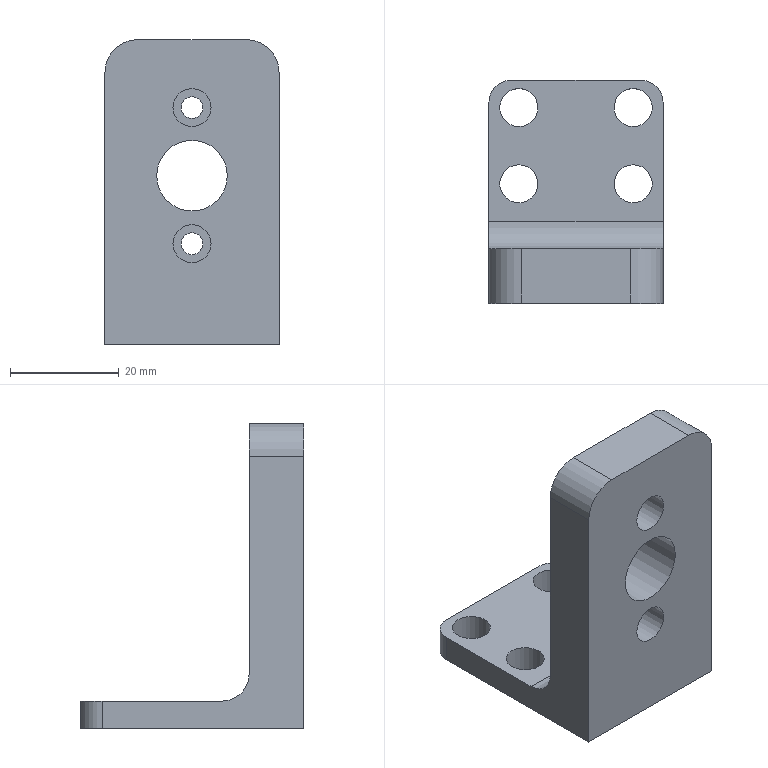Part | NX | features BREP 1, DATUM_CSYS 1 | 1 solid | 30 faces | box 32 x 41 x 56 mm | volume 19804 mm3 | cylinder 18 | plane 10 | cone 2 | commonest cylinder face diameters 7 x6 4.2 x4 4 x2 8 x2 12 x2 10 x1
STEP:
#1=CARTESIAN_POINT('',(-16.,0.,-28.));
#2=VERTEX_POINT('',#1);
#3=CARTESIAN_POINT('',(16.,0.,-28.));
#4=VERTEX_POINT('',#3);
#5=CARTESIAN_POINT('',(-16.,0.,-28.));
#6=DIRECTION('',(1.,0.,0.));
#7=VECTOR('',#6,1000.);
#8=LINE('',#5,#7);
#9=EDGE_CURVE('',#2,#4,#8,.T.);
#10=ORIENTED_EDGE('',*,*,#9,.T.);
#11=CARTESIAN_POINT('',(16.,0.,22.));
#12=VERTEX_POINT('',#11);
#13=CARTESIAN_POINT('',(16.,0.,-28.));
#14=DIRECTION('',(0.,0.,1.));
#15=VECTOR('',#14,1000.);
#16=LINE('',#13,#15);
#17=EDGE_CURVE('',#4,#12,#16,.T.);
#18=ORIENTED_EDGE('',*,*,#17,.T.);
#19=CARTESIAN_POINT('',(10.,0.,28.));
#20=VERTEX_POINT('',#19);
#21=CARTESIAN_POINT('',(10.,0.,22.));
#22=DIRECTION('',(0.,-1.,0.));
#23=DIRECTION('',(1.,0.,0.));
#24=AXIS2_PLACEMENT_3D('',#21,#22,#23);
#25=CIRCLE('',#24,6.);
#26=EDGE_CURVE('',#12,#20,#25,.T.);
#27=ORIENTED_EDGE('',*,*,#26,.T.);
#28=CARTESIAN_POINT('',(-10.,0.,28.));
#29=VERTEX_POINT('',#28);
#30=CARTESIAN_POINT('',(10.,0.,28.));
#31=DIRECTION('',(-1.,0.,0.));
#32=VECTOR('',#31,1000.);
#33=LINE('',#30,#32);
#34=EDGE_CURVE('',#20,#29,#33,.T.);
#35=ORIENTED_EDGE('',*,*,#34,.T.);
#36=CARTESIAN_POINT('',(-16.,0.,22.));
#37=VERTEX_POINT('',#36);
#38=CARTESIAN_POINT('',(-10.,0.,22.));
#39=DIRECTION('',(0.,-1.,0.));
#40=DIRECTION('',(0.,0.,1.));
#41=AXIS2_PLACEMENT_3D('',#38,#39,#40);
#42=CIRCLE('',#41,6.);
#43=EDGE_CURVE('',#29,#37,#42,.T.);
#44=ORIENTED_EDGE('',*,*,#43,.T.);
#45=CARTESIAN_POINT('',(-16.,0.,22.));
#46=DIRECTION('',(0.,0.,-1.));
#47=VECTOR('',#46,1000.);
#48=LINE('',#45,#47);
#49=EDGE_CURVE('',#37,#2,#48,.T.);
#50=ORIENTED_EDGE('',*,*,#49,.T.);
#51=EDGE_LOOP('',(#10,#18,#27,#35,#44,#50));
#52=FACE_BOUND('',#51,.T.);
#53=CARTESIAN_POINT('',(3.5,0.,15.5));
#54=VERTEX_POINT('',#53);
#55=CARTESIAN_POINT('',(0.,0.,15.5));
#56=DIRECTION('',(0.,1.,0.));
#57=DIRECTION('',(1.,0.,0.));
#58=AXIS2_PLACEMENT_3D('',#55,#56,#57);
#59=CIRCLE('',#58,3.5);
#60=EDGE_CURVE('',#54,#54,#59,.T.);
#61=ORIENTED_EDGE('',*,*,#60,.T.);
#62=EDGE_LOOP('',(#61));
#63=FACE_BOUND('',#62,.T.);
#64=CARTESIAN_POINT('',(6.5,0.,3.));
#65=VERTEX_POINT('',#64);
#66=CARTESIAN_POINT('',(0.,0.,3.));
#67=DIRECTION('',(0.,1.,0.));
#68=DIRECTION('',(1.,0.,0.));
#69=AXIS2_PLACEMENT_3D('',#66,#67,#68);
#70=CIRCLE('',#69,6.5);
#71=EDGE_CURVE('',#65,#65,#70,.T.);
#72=ORIENTED_EDGE('',*,*,#71,.T.);
#73=EDGE_LOOP('',(#72));
#74=FACE_BOUND('',#73,.T.);
#75=CARTESIAN_POINT('',(3.5,0.,-9.5));
#76=VERTEX_POINT('',#75);
#77=CARTESIAN_POINT('',(0.,0.,-9.5));
#78=DIRECTION('',(0.,1.,0.));
#79=DIRECTION('',(1.,0.,0.));
#80=AXIS2_PLACEMENT_3D('',#77,#78,#79);
#81=CIRCLE('',#80,3.5);
#82=EDGE_CURVE('',#76,#76,#81,.T.);
#83=ORIENTED_EDGE('',*,*,#82,.T.);
#84=EDGE_LOOP('',(#83));
#85=FACE_BOUND('',#84,.T.);
#86=CARTESIAN_POINT('',(8.143,0.,0.));
#87=DIRECTION('',(0.,-1.,0.));
#88=DIRECTION('',(-1.,0.,0.));
#89=AXIS2_PLACEMENT_3D('',#86,#87,#88);
#90=PLANE('',#89);
#91=ADVANCED_FACE('',(#52,#63,#74,#85),#90,.T.);
#92=CARTESIAN_POINT('',(16.,10.,-18.));
#93=VERTEX_POINT('',#92);
#94=CARTESIAN_POINT('',(16.,10.,22.));
#95=VERTEX_POINT('',#94);
#96=CARTESIAN_POINT('',(16.,10.,-18.));
#97=DIRECTION('',(0.,0.,1.));
#98=VECTOR('',#97,1000.);
#99=LINE('',#96,#98);
#100=EDGE_CURVE('',#93,#95,#99,.T.);
#101=ORIENTED_EDGE('',*,*,#100,.F.);
#102=CARTESIAN_POINT('',(-16.,10.,-18.));
#103=VERTEX_POINT('',#102);
#104=CARTESIAN_POINT('',(16.,10.,-18.));
#105=DIRECTION('',(-1.,0.,0.));
#106=VECTOR('',#105,1000.);
#107=LINE('',#104,#106);
#108=EDGE_CURVE('',#93,#103,#107,.T.);
#109=ORIENTED_EDGE('',*,*,#108,.T.);
#110=CARTESIAN_POINT('',(-16.,10.,22.));
#111=VERTEX_POINT('',#110);
#112=CARTESIAN_POINT('',(-16.,10.,22.));
#113=DIRECTION('',(0.,0.,-1.));
#114=VECTOR('',#113,1000.);
#115=LINE('',#112,#114);
#116=EDGE_CURVE('',#111,#103,#115,.T.);
#117=ORIENTED_EDGE('',*,*,#116,.F.);
#118=CARTESIAN_POINT('',(-10.,10.,28.));
#119=VERTEX_POINT('',#118);
#120=CARTESIAN_POINT('',(-10.,10.,22.));
#121=DIRECTION('',(0.,-1.,0.));
#122=DIRECTION('',(0.,0.,1.));
#123=AXIS2_PLACEMENT_3D('',#120,#121,#122);
#124=CIRCLE('',#123,6.);
#125=EDGE_CURVE('',#119,#111,#124,.T.);
#126=ORIENTED_EDGE('',*,*,#125,.F.);
#127=CARTESIAN_POINT('',(10.,10.,28.));
#128=VERTEX_POINT('',#127);
#129=CARTESIAN_POINT('',(10.,10.,28.));
#130=DIRECTION('',(-1.,0.,0.));
#131=VECTOR('',#130,1000.);
#132=LINE('',#129,#131);
#133=EDGE_CURVE('',#128,#119,#132,.T.);
#134=ORIENTED_EDGE('',*,*,#133,.F.);
#135=CARTESIAN_POINT('',(10.,10.,22.));
#136=DIRECTION('',(0.,-1.,0.));
#137=DIRECTION('',(1.,0.,0.));
#138=AXIS2_PLACEMENT_3D('',#135,#136,#137);
#139=CIRCLE('',#138,6.);
#140=EDGE_CURVE('',#95,#128,#139,.T.);
#141=ORIENTED_EDGE('',*,*,#140,.F.);
#142=EDGE_LOOP('',(#101,#109,#117,#126,#134,#141));
#143=FACE_BOUND('',#142,.T.);
#144=CARTESIAN_POINT('',(6.5,10.,3.));
#145=VERTEX_POINT('',#144);
#146=CARTESIAN_POINT('',(0.,10.,3.));
#147=DIRECTION('',(0.,1.,0.));
#148=DIRECTION('',(1.,0.,0.));
#149=AXIS2_PLACEMENT_3D('',#146,#147,#148);
#150=CIRCLE('',#149,6.5);
#151=EDGE_CURVE('',#145,#145,#150,.T.);
#152=ORIENTED_EDGE('',*,*,#151,.F.);
#153=EDGE_LOOP('',(#152));
#154=FACE_BOUND('',#153,.T.);
#155=CARTESIAN_POINT('',(2.,10.,-9.5));
#156=VERTEX_POINT('',#155);
#157=CARTESIAN_POINT('',(0.,10.,-9.5));
#158=DIRECTION('',(0.,1.,0.));
#159=DIRECTION('',(1.,0.,0.));
#160=AXIS2_PLACEMENT_3D('',#157,#158,#159);
#161=CIRCLE('',#160,2.);
#162=EDGE_CURVE('',#156,#156,#161,.T.);
#163=ORIENTED_EDGE('',*,*,#162,.F.);
#164=EDGE_LOOP('',(#163));
#165=FACE_BOUND('',#164,.T.);
#166=CARTESIAN_POINT('',(2.,10.,15.5));
#167=VERTEX_POINT('',#166);
#168=CARTESIAN_POINT('',(0.,10.,15.5));
#169=DIRECTION('',(0.,1.,0.));
#170=DIRECTION('',(1.,0.,0.));
#171=AXIS2_PLACEMENT_3D('',#168,#169,#170);
#172=CIRCLE('',#171,2.);
#173=EDGE_CURVE('',#167,#167,#172,.T.);
#174=ORIENTED_EDGE('',*,*,#173,.F.);
#175=EDGE_LOOP('',(#174));
#176=FACE_BOUND('',#175,.T.);
#177=CARTESIAN_POINT('',(8.143,10.,0.));
#178=DIRECTION('',(0.,-1.,0.));
#179=DIRECTION('',(-1.,0.,0.));
#180=AXIS2_PLACEMENT_3D('',#177,#178,#179);
#181=PLANE('',#180);
#182=ADVANCED_FACE('',(#143,#154,#165,#176),#181,.F.);
#183=CARTESIAN_POINT('',(-16.,37.,-28.));
#184=VERTEX_POINT('',#183);
#185=CARTESIAN_POINT('',(-16.,0.,-28.));
#186=DIRECTION('',(0.,1.,0.));
#187=VECTOR('',#186,1000.);
#188=LINE('',#185,#187);
#189=EDGE_CURVE('',#2,#184,#188,.T.);
#190=ORIENTED_EDGE('',*,*,#189,.T.);
#191=CARTESIAN_POINT('',(-12.,41.,-28.));
#192=VERTEX_POINT('',#191);
#193=CARTESIAN_POINT('',(-12.,37.,-28.));
#194=DIRECTION('',(0.,0.,-1.));
#195=DIRECTION('',(-1.,0.,0.));
#196=AXIS2_PLACEMENT_3D('',#193,#194,#195);
#197=CIRCLE('',#196,4.);
#198=EDGE_CURVE('',#184,#192,#197,.T.);
#199=ORIENTED_EDGE('',*,*,#198,.T.);
#200=CARTESIAN_POINT('',(12.,41.,-28.));
#201=VERTEX_POINT('',#200);
#202=CARTESIAN_POINT('',(12.,41.,-28.));
#203=DIRECTION('',(-1.,0.,0.));
#204=VECTOR('',#203,1000.);
#205=LINE('',#202,#204);
#206=EDGE_CURVE('',#201,#192,#205,.T.);
#207=ORIENTED_EDGE('',*,*,#206,.F.);
#208=CARTESIAN_POINT('',(16.,37.,-28.));
#209=VERTEX_POINT('',#208);
#210=CARTESIAN_POINT('',(12.,37.,-28.));
#211=DIRECTION('',(0.,0.,1.));
#212=DIRECTION('',(1.,0.,0.));
#213=AXIS2_PLACEMENT_3D('',#210,#211,#212);
#214=CIRCLE('',#213,4.);
#215=EDGE_CURVE('',#209,#201,#214,.T.);
#216=ORIENTED_EDGE('',*,*,#215,.F.);
#217=CARTESIAN_POINT('',(16.,0.,-28.));
#218=DIRECTION('',(0.,1.,0.));
#219=VECTOR('',#218,1000.);
#220=LINE('',#217,#219);
#221=EDGE_CURVE('',#4,#209,#220,.T.);
#222=ORIENTED_EDGE('',*,*,#221,.F.);
#223=ORIENTED_EDGE('',*,*,#9,.F.);
#224=EDGE_LOOP('',(#190,#199,#207,#216,#222,#223));
#225=FACE_BOUND('',#224,.T.);
#226=CARTESIAN_POINT('',(10.5,39.5,-28.));
#227=VERTEX_POINT('',#226);
#228=CARTESIAN_POINT('',(10.5,36.,-28.));
#229=DIRECTION('',(0.,0.,-1.));
#230=DIRECTION('',(0.,1.,0.));
#231=AXIS2_PLACEMENT_3D('',#228,#229,#230);
#232=CIRCLE('',#231,3.5);
#233=EDGE_CURVE('',#227,#227,#232,.T.);
#234=ORIENTED_EDGE('',*,*,#233,.F.);
#235=EDGE_LOOP('',(#234));
#236=FACE_BOUND('',#235,.T.);
#237=CARTESIAN_POINT('',(-10.5,39.5,-28.));
#238=VERTEX_POINT('',#237);
#239=CARTESIAN_POINT('',(-10.5,36.,-28.));
#240=DIRECTION('',(0.,0.,-1.));
#241=DIRECTION('',(0.,1.,0.));
#242=AXIS2_PLACEMENT_3D('',#239,#240,#241);
#243=CIRCLE('',#242,3.5);
#244=EDGE_CURVE('',#238,#238,#243,.T.);
#245=ORIENTED_EDGE('',*,*,#244,.F.);
#246=EDGE_LOOP('',(#245));
#247=FACE_BOUND('',#246,.T.);
#248=CARTESIAN_POINT('',(10.5,25.5,-28.));
#249=VERTEX_POINT('',#248);
#250=CARTESIAN_POINT('',(10.5,22.,-28.));
#251=DIRECTION('',(0.,0.,-1.));
#252=DIRECTION('',(0.,1.,0.));
#253=AXIS2_PLACEMENT_3D('',#250,#251,#252);
#254=CIRCLE('',#253,3.5);
#255=EDGE_CURVE('',#249,#249,#254,.T.);
#256=ORIENTED_EDGE('',*,*,#255,.F.);
#257=EDGE_LOOP('',(#256));
#258=FACE_BOUND('',#257,.T.);
#259=CARTESIAN_POINT('',(-10.5,25.5,-28.));
#260=VERTEX_POINT('',#259);
#261=CARTESIAN_POINT('',(-10.5,22.,-28.));
#262=DIRECTION('',(0.,0.,-1.));
#263=DIRECTION('',(0.,1.,0.));
#264=AXIS2_PLACEMENT_3D('',#261,#262,#263);
#265=CIRCLE('',#264,3.5);
#266=EDGE_CURVE('',#260,#260,#265,.T.);
#267=ORIENTED_EDGE('',*,*,#266,.F.);
#268=EDGE_LOOP('',(#267));
#269=FACE_BOUND('',#268,.T.);
#270=CARTESIAN_POINT('',(-7.9,5.,-28.));
#271=VERTEX_POINT('',#270);
#272=CARTESIAN_POINT('',(-10.,5.,-28.));
#273=DIRECTION('',(0.,0.,1.));
#274=DIRECTION('',(1.,0.,0.));
#275=AXIS2_PLACEMENT_3D('',#272,#273,#274);
#276=CIRCLE('',#275,2.1);
#277=EDGE_CURVE('',#271,#271,#276,.T.);
#278=ORIENTED_EDGE('',*,*,#277,.T.);
#279=EDGE_LOOP('',(#278));
#280=FACE_BOUND('',#279,.T.);
#281=CARTESIAN_POINT('',(12.1,5.,-28.));
#282=VERTEX_POINT('',#281);
#283=CARTESIAN_POINT('',(10.,5.,-28.));
#284=DIRECTION('',(0.,0.,1.));
#285=DIRECTION('',(1.,0.,0.));
#286=AXIS2_PLACEMENT_3D('',#283,#284,#285);
#287=CIRCLE('',#286,2.1);
#288=EDGE_CURVE('',#282,#282,#287,.T.);
#289=ORIENTED_EDGE('',*,*,#288,.T.);
#290=EDGE_LOOP('',(#289));
#291=FACE_BOUND('',#290,.T.);
#292=CARTESIAN_POINT('',(0.,20.5,-28.));
#293=DIRECTION('',(0.,0.,1.));
#294=DIRECTION('',(-1.,0.,0.));
#295=AXIS2_PLACEMENT_3D('',#292,#293,#294);
#296=PLANE('',#295);
#297=ADVANCED_FACE('',(#225,#236,#247,#258,#269,#280,#291),#296,.F.);
#298=CARTESIAN_POINT('',(16.,37.,-23.));
#299=VERTEX_POINT('',#298);
#300=CARTESIAN_POINT('',(16.,37.,-28.));
#301=DIRECTION('',(0.,0.,1.));
#302=VECTOR('',#301,1000.);
#303=LINE('',#300,#302);
#304=EDGE_CURVE('',#209,#299,#303,.T.);
#305=ORIENTED_EDGE('',*,*,#304,.T.);
#306=CARTESIAN_POINT('',(16.,15.,-23.));
#307=VERTEX_POINT('',#306);
#308=CARTESIAN_POINT('',(16.,37.,-23.));
#309=DIRECTION('',(0.,-1.,0.));
#310=VECTOR('',#309,1000.);
#311=LINE('',#308,#310);
#312=EDGE_CURVE('',#299,#307,#311,.T.);
#313=ORIENTED_EDGE('',*,*,#312,.T.);
#314=CARTESIAN_POINT('',(16.,15.,-18.));
#315=DIRECTION('',(-1.,0.,0.));
#316=DIRECTION('',(0.,0.,-1.));
#317=AXIS2_PLACEMENT_3D('',#314,#315,#316);
#318=CIRCLE('',#317,5.);
#319=EDGE_CURVE('',#307,#93,#318,.T.);
#320=ORIENTED_EDGE('',*,*,#319,.T.);
#321=ORIENTED_EDGE('',*,*,#100,.T.);
#322=CARTESIAN_POINT('',(16.,0.,22.));
#323=DIRECTION('',(0.,1.,0.));
#324=VECTOR('',#323,1000.);
#325=LINE('',#322,#324);
#326=EDGE_CURVE('',#12,#95,#325,.T.);
#327=ORIENTED_EDGE('',*,*,#326,.F.);
#328=ORIENTED_EDGE('',*,*,#17,.F.);
#329=ORIENTED_EDGE('',*,*,#221,.T.);
#330=EDGE_LOOP('',(#305,#313,#320,#321,#327,#328,#329));
#331=FACE_BOUND('',#330,.T.);
#332=CARTESIAN_POINT('',(16.,21.275,-3.775));
#333=DIRECTION('',(-1.,0.,0.));
#334=DIRECTION('',(0.,0.,-1.));
#335=AXIS2_PLACEMENT_3D('',#332,#333,#334);
#336=PLANE('',#335);
#337=ADVANCED_FACE('',(#331),#336,.F.);
#338=ORIENTED_EDGE('',*,*,#326,.T.);
#339=ORIENTED_EDGE('',*,*,#140,.T.);
#340=CARTESIAN_POINT('',(10.,0.,28.));
#341=DIRECTION('',(0.,1.,0.));
#342=VECTOR('',#341,1000.);
#343=LINE('',#340,#342);
#344=EDGE_CURVE('',#20,#128,#343,.T.);
#345=ORIENTED_EDGE('',*,*,#344,.F.);
#346=ORIENTED_EDGE('',*,*,#26,.F.);
#347=EDGE_LOOP('',(#338,#339,#345,#346));
#348=FACE_BOUND('',#347,.T.);
#349=CARTESIAN_POINT('',(10.,0.,22.));
#350=DIRECTION('',(0.,1.,0.));
#351=DIRECTION('',(-1.,0.,0.));
#352=AXIS2_PLACEMENT_3D('',#349,#350,#351);
#353=CYLINDRICAL_SURFACE('',#352,6.);
#354=ADVANCED_FACE('',(#348),#353,.T.);
#355=ORIENTED_EDGE('',*,*,#344,.T.);
#356=ORIENTED_EDGE('',*,*,#133,.T.);
#357=CARTESIAN_POINT('',(-10.,0.,28.));
#358=DIRECTION('',(0.,1.,0.));
#359=VECTOR('',#358,1000.);
#360=LINE('',#357,#359);
#361=EDGE_CURVE('',#29,#119,#360,.T.);
#362=ORIENTED_EDGE('',*,*,#361,.F.);
#363=ORIENTED_EDGE('',*,*,#34,.F.);
#364=EDGE_LOOP('',(#355,#356,#362,#363));
#365=FACE_BOUND('',#364,.T.);
#366=CARTESIAN_POINT('',(0.,5.,28.));
#367=DIRECTION('',(0.,0.,-1.));
#368=DIRECTION('',(1.,0.,0.));
#369=AXIS2_PLACEMENT_3D('',#366,#367,#368);
#370=PLANE('',#369);
#371=ADVANCED_FACE('',(#365),#370,.F.);
#372=ORIENTED_EDGE('',*,*,#361,.T.);
#373=ORIENTED_EDGE('',*,*,#125,.T.);
#374=CARTESIAN_POINT('',(-16.,0.,22.));
#375=DIRECTION('',(0.,1.,0.));
#376=VECTOR('',#375,1000.);
#377=LINE('',#374,#376);
#378=EDGE_CURVE('',#37,#111,#377,.T.);
#379=ORIENTED_EDGE('',*,*,#378,.F.);
#380=ORIENTED_EDGE('',*,*,#43,.F.);
#381=EDGE_LOOP('',(#372,#373,#379,#380));
#382=FACE_BOUND('',#381,.T.);
#383=CARTESIAN_POINT('',(-10.,0.,22.));
#384=DIRECTION('',(0.,1.,0.));
#385=DIRECTION('',(0.,0.,-1.));
#386=AXIS2_PLACEMENT_3D('',#383,#384,#385);
#387=CYLINDRICAL_SURFACE('',#386,6.);
#388=ADVANCED_FACE('',(#382),#387,.T.);
#389=CARTESIAN_POINT('',(-16.,15.,-23.));
#390=VERTEX_POINT('',#389);
#391=CARTESIAN_POINT('',(-16.,15.,-18.));
#392=DIRECTION('',(-1.,0.,0.));
#393=DIRECTION('',(0.,0.,-1.));
#394=AXIS2_PLACEMENT_3D('',#391,#392,#393);
#395=CIRCLE('',#394,5.);
#396=EDGE_CURVE('',#390,#103,#395,.T.);
#397=ORIENTED_EDGE('',*,*,#396,.F.);
#398=CARTESIAN_POINT('',(-16.,37.,-23.));
#399=VERTEX_POINT('',#398);
#400=CARTESIAN_POINT('',(-16.,37.,-23.));
#401=DIRECTION('',(0.,-1.,0.));
#402=VECTOR('',#401,1000.);
#403=LINE('',#400,#402);
#404=EDGE_CURVE('',#399,#390,#403,.T.);
#405=ORIENTED_EDGE('',*,*,#404,.F.);
#406=CARTESIAN_POINT('',(-16.,37.,-28.));
#407=DIRECTION('',(0.,0.,1.));
#408=VECTOR('',#407,1000.);
#409=LINE('',#406,#408);
#410=EDGE_CURVE('',#184,#399,#409,.T.);
#411=ORIENTED_EDGE('',*,*,#410,.F.);
#412=ORIENTED_EDGE('',*,*,#189,.F.);
#413=ORIENTED_EDGE('',*,*,#49,.F.);
#414=ORIENTED_EDGE('',*,*,#378,.T.);
#415=ORIENTED_EDGE('',*,*,#116,.T.);
#416=EDGE_LOOP('',(#397,#405,#411,#412,#413,#414,#415));
#417=FACE_BOUND('',#416,.T.);
#418=CARTESIAN_POINT('',(-16.,21.275,-3.775));
#419=DIRECTION('',(1.,0.,0.));
#420=DIRECTION('',(0.,0.,1.));
#421=AXIS2_PLACEMENT_3D('',#418,#419,#420);
#422=PLANE('',#421);
#423=ADVANCED_FACE('',(#417),#422,.F.);
#424=CARTESIAN_POINT('',(6.5,0.,3.));
#425=DIRECTION('',(0.,1.,0.));
#426=VECTOR('',#425,1000.);
#427=LINE('',#424,#426);
#428=EDGE_CURVE('',#65,#145,#427,.T.);
#429=ORIENTED_EDGE('',*,*,#428,.T.);
#430=ORIENTED_EDGE('',*,*,#151,.T.);
#431=ORIENTED_EDGE('',*,*,#428,.F.);
#432=ORIENTED_EDGE('',*,*,#71,.F.);
#433=EDGE_LOOP('',(#429,#430,#431,#432));
#434=FACE_BOUND('',#433,.T.);
#435=CARTESIAN_POINT('',(0.,0.,3.));
#436=DIRECTION('',(0.,1.,0.));
#437=DIRECTION('',(-1.,0.,0.));
#438=AXIS2_PLACEMENT_3D('',#435,#436,#437);
#439=CYLINDRICAL_SURFACE('',#438,6.5);
#440=ADVANCED_FACE('',(#434),#439,.F.);
#441=ORIENTED_EDGE('',*,*,#162,.T.);
#442=CARTESIAN_POINT('',(2.,6.,-9.5));
#443=VERTEX_POINT('',#442);
#444=CARTESIAN_POINT('',(2.,6.,-9.5));
#445=DIRECTION('',(0.,1.,0.));
#446=VECTOR('',#445,1000.);
#447=LINE('',#444,#446);
#448=EDGE_CURVE('',#443,#156,#447,.T.);
#449=ORIENTED_EDGE('',*,*,#448,.F.);
#450=CARTESIAN_POINT('',(0.,6.,-9.5));
#451=DIRECTION('',(0.,1.,0.));
#452=DIRECTION('',(1.,0.,0.));
#453=AXIS2_PLACEMENT_3D('',#450,#451,#452);
#454=CIRCLE('',#453,2.);
#455=EDGE_CURVE('',#443,#443,#454,.T.);
#456=ORIENTED_EDGE('',*,*,#455,.F.);
#457=ORIENTED_EDGE('',*,*,#448,.T.);
#458=EDGE_LOOP('',(#441,#449,#456,#457));
#459=FACE_BOUND('',#458,.T.);
#460=CARTESIAN_POINT('',(0.,0.,-9.5));
#461=DIRECTION('',(0.,1.,0.));
#462=DIRECTION('',(-1.,0.,0.));
#463=AXIS2_PLACEMENT_3D('',#460,#461,#462);
#464=CYLINDRICAL_SURFACE('',#463,2.);
#465=ADVANCED_FACE('',(#459),#464,.F.);
#466=ORIENTED_EDGE('',*,*,#173,.T.);
#467=CARTESIAN_POINT('',(2.,6.,15.5));
#468=VERTEX_POINT('',#467);
#469=CARTESIAN_POINT('',(2.,6.,15.5));
#470=DIRECTION('',(0.,1.,0.));
#471=VECTOR('',#470,1000.);
#472=LINE('',#469,#471);
#473=EDGE_CURVE('',#468,#167,#472,.T.);
#474=ORIENTED_EDGE('',*,*,#473,.F.);
#475=CARTESIAN_POINT('',(0.,6.,15.5));
#476=DIRECTION('',(0.,1.,0.));
#477=DIRECTION('',(1.,0.,0.));
#478=AXIS2_PLACEMENT_3D('',#475,#476,#477);
#479=CIRCLE('',#478,2.);
#480=EDGE_CURVE('',#468,#468,#479,.T.);
#481=ORIENTED_EDGE('',*,*,#480,.F.);
#482=ORIENTED_EDGE('',*,*,#473,.T.);
#483=EDGE_LOOP('',(#466,#474,#481,#482));
#484=FACE_BOUND('',#483,.T.);
#485=CARTESIAN_POINT('',(0.,0.,15.5));
#486=DIRECTION('',(0.,1.,0.));
#487=DIRECTION('',(-1.,0.,0.));
#488=AXIS2_PLACEMENT_3D('',#485,#486,#487);
#489=CYLINDRICAL_SURFACE('',#488,2.);
#490=ADVANCED_FACE('',(#484),#489,.F.);
#491=CARTESIAN_POINT('',(3.5,6.,15.5));
#492=VERTEX_POINT('',#491);
#493=CARTESIAN_POINT('',(0.,6.,15.5));
#494=DIRECTION('',(0.,1.,0.));
#495=DIRECTION('',(1.,0.,0.));
#496=AXIS2_PLACEMENT_3D('',#493,#494,#495);
#497=CIRCLE('',#496,3.5);
#498=EDGE_CURVE('',#492,#492,#497,.T.);
#499=ORIENTED_EDGE('',*,*,#498,.F.);
#500=EDGE_LOOP('',(#499));
#501=FACE_BOUND('',#500,.T.);
#502=ORIENTED_EDGE('',*,*,#480,.T.);
#503=EDGE_LOOP('',(#502));
#504=FACE_BOUND('',#503,.T.);
#505=CARTESIAN_POINT('',(0.,6.,15.5));
#506=DIRECTION('',(0.,1.,0.));
#507=DIRECTION('',(-1.,0.,0.));
#508=AXIS2_PLACEMENT_3D('',#505,#506,#507);
#509=PLANE('',#508);
#510=ADVANCED_FACE('',(#501,#504),#509,.F.);
#511=CARTESIAN_POINT('',(3.5,0.,15.5));
#512=DIRECTION('',(0.,1.,0.));
#513=VECTOR('',#512,1000.);
#514=LINE('',#511,#513);
#515=EDGE_CURVE('',#54,#492,#514,.T.);
#516=ORIENTED_EDGE('',*,*,#515,.T.);
#517=ORIENTED_EDGE('',*,*,#498,.T.);
#518=ORIENTED_EDGE('',*,*,#515,.F.);
#519=ORIENTED_EDGE('',*,*,#60,.F.);
#520=EDGE_LOOP('',(#516,#517,#518,#519));
#521=FACE_BOUND('',#520,.T.);
#522=CARTESIAN_POINT('',(0.,0.,15.5));
#523=DIRECTION('',(0.,1.,0.));
#524=DIRECTION('',(-1.,0.,0.));
#525=AXIS2_PLACEMENT_3D('',#522,#523,#524);
#526=CYLINDRICAL_SURFACE('',#525,3.5);
#527=ADVANCED_FACE('',(#521),#526,.F.);
#528=CARTESIAN_POINT('',(3.5,6.,-9.5));
#529=VERTEX_POINT('',#528);
#530=CARTESIAN_POINT('',(0.,6.,-9.5));
#531=DIRECTION('',(0.,1.,0.));
#532=DIRECTION('',(1.,0.,0.));
#533=AXIS2_PLACEMENT_3D('',#530,#531,#532);
#534=CIRCLE('',#533,3.5);
#535=EDGE_CURVE('',#529,#529,#534,.T.);
#536=ORIENTED_EDGE('',*,*,#535,.F.);
#537=EDGE_LOOP('',(#536));
#538=FACE_BOUND('',#537,.T.);
#539=ORIENTED_EDGE('',*,*,#455,.T.);
#540=EDGE_LOOP('',(#539));
#541=FACE_BOUND('',#540,.T.);
#542=CARTESIAN_POINT('',(0.,6.,-9.5));
#543=DIRECTION('',(0.,1.,0.));
#544=DIRECTION('',(-1.,0.,0.));
#545=AXIS2_PLACEMENT_3D('',#542,#543,#544);
#546=PLANE('',#545);
#547=ADVANCED_FACE('',(#538,#541),#546,.F.);
#548=CARTESIAN_POINT('',(3.5,0.,-9.5));
#549=DIRECTION('',(0.,1.,0.));
#550=VECTOR('',#549,1000.);
#551=LINE('',#548,#550);
#552=EDGE_CURVE('',#76,#529,#551,.T.);
#553=ORIENTED_EDGE('',*,*,#552,.T.);
#554=ORIENTED_EDGE('',*,*,#535,.T.);
#555=ORIENTED_EDGE('',*,*,#552,.F.);
#556=ORIENTED_EDGE('',*,*,#82,.F.);
#557=EDGE_LOOP('',(#553,#554,#555,#556));
#558=FACE_BOUND('',#557,.T.);
#559=CARTESIAN_POINT('',(0.,0.,-9.5));
#560=DIRECTION('',(0.,1.,0.));
#561=DIRECTION('',(-1.,0.,0.));
#562=AXIS2_PLACEMENT_3D('',#559,#560,#561);
#563=CYLINDRICAL_SURFACE('',#562,3.5);
#564=ADVANCED_FACE('',(#558),#563,.F.);
#565=CARTESIAN_POINT('',(12.,41.,-23.));
#566=VERTEX_POINT('',#565);
#567=CARTESIAN_POINT('',(12.,41.,-28.));
#568=DIRECTION('',(0.,0.,1.));
#569=VECTOR('',#568,1000.);
#570=LINE('',#567,#569);
#571=EDGE_CURVE('',#201,#566,#570,.T.);
#572=ORIENTED_EDGE('',*,*,#571,.F.);
#573=ORIENTED_EDGE('',*,*,#206,.T.);
#574=CARTESIAN_POINT('',(-12.,41.,-23.));
#575=VERTEX_POINT('',#574);
#576=CARTESIAN_POINT('',(-12.,41.,-28.));
#577=DIRECTION('',(0.,0.,1.));
#578=VECTOR('',#577,1000.);
#579=LINE('',#576,#578);
#580=EDGE_CURVE('',#192,#575,#579,.T.);
#581=ORIENTED_EDGE('',*,*,#580,.T.);
#582=CARTESIAN_POINT('',(12.,41.,-23.));
#583=DIRECTION('',(-1.,0.,0.));
#584=VECTOR('',#583,1000.);
#585=LINE('',#582,#584);
#586=EDGE_CURVE('',#566,#575,#585,.T.);
#587=ORIENTED_EDGE('',*,*,#586,.F.);
#588=EDGE_LOOP('',(#572,#573,#581,#587));
#589=FACE_BOUND('',#588,.T.);
#590=CARTESIAN_POINT('',(0.,41.,-25.5));
#591=DIRECTION('',(0.,-1.,0.));
#592=DIRECTION('',(0.,0.,-1.));
#593=AXIS2_PLACEMENT_3D('',#590,#591,#592);
#594=PLANE('',#593);
#595=ADVANCED_FACE('',(#589),#594,.F.);
#596=ORIENTED_EDGE('',*,*,#312,.F.);
#597=CARTESIAN_POINT('',(12.,37.,-23.));
#598=DIRECTION('',(0.,0.,1.));
#599=DIRECTION('',(1.,0.,0.));
#600=AXIS2_PLACEMENT_3D('',#597,#598,#599);
#601=CIRCLE('',#600,4.);
#602=EDGE_CURVE('',#299,#566,#601,.T.);
#603=ORIENTED_EDGE('',*,*,#602,.T.);
#604=ORIENTED_EDGE('',*,*,#586,.T.);
#605=CARTESIAN_POINT('',(-12.,37.,-23.));
#606=DIRECTION('',(0.,0.,-1.));
#607=DIRECTION('',(-1.,0.,0.));
#608=AXIS2_PLACEMENT_3D('',#605,#606,#607);
#609=CIRCLE('',#608,4.);
#610=EDGE_CURVE('',#399,#575,#609,.T.);
#611=ORIENTED_EDGE('',*,*,#610,.F.);
#612=ORIENTED_EDGE('',*,*,#404,.T.);
#613=CARTESIAN_POINT('',(16.,15.,-23.));
#614=DIRECTION('',(-1.,0.,0.));
#615=VECTOR('',#614,1000.);
#616=LINE('',#613,#615);
#617=EDGE_CURVE('',#307,#390,#616,.T.);
#618=ORIENTED_EDGE('',*,*,#617,.F.);
#619=EDGE_LOOP('',(#596,#603,#604,#611,#612,#618));
#620=FACE_BOUND('',#619,.T.);
#621=CARTESIAN_POINT('',(-10.5,25.5,-23.));
#622=VERTEX_POINT('',#621);
#623=CARTESIAN_POINT('',(-10.5,22.,-23.));
#624=DIRECTION('',(0.,0.,1.));
#625=DIRECTION('',(0.,1.,0.));
#626=AXIS2_PLACEMENT_3D('',#623,#624,#625);
#627=CIRCLE('',#626,3.5);
#628=EDGE_CURVE('',#622,#622,#627,.T.);
#629=ORIENTED_EDGE('',*,*,#628,.F.);
#630=EDGE_LOOP('',(#629));
#631=FACE_BOUND('',#630,.T.);
#632=CARTESIAN_POINT('',(10.5,25.5,-23.));
#633=VERTEX_POINT('',#632);
#634=CARTESIAN_POINT('',(10.5,22.,-23.));
#635=DIRECTION('',(0.,0.,1.));
#636=DIRECTION('',(0.,1.,0.));
#637=AXIS2_PLACEMENT_3D('',#634,#635,#636);
#638=CIRCLE('',#637,3.5);
#639=EDGE_CURVE('',#633,#633,#638,.T.);
#640=ORIENTED_EDGE('',*,*,#639,.F.);
#641=EDGE_LOOP('',(#640));
#642=FACE_BOUND('',#641,.T.);
#643=CARTESIAN_POINT('',(-10.5,39.5,-23.));
#644=VERTEX_POINT('',#643);
#645=CARTESIAN_POINT('',(-10.5,36.,-23.));
#646=DIRECTION('',(0.,0.,1.));
#647=DIRECTION('',(0.,1.,0.));
#648=AXIS2_PLACEMENT_3D('',#645,#646,#647);
#649=CIRCLE('',#648,3.5);
#650=EDGE_CURVE('',#644,#644,#649,.T.);
#651=ORIENTED_EDGE('',*,*,#650,.F.);
#652=EDGE_LOOP('',(#651));
#653=FACE_BOUND('',#652,.T.);
#654=CARTESIAN_POINT('',(10.5,39.5,-23.));
#655=VERTEX_POINT('',#654);
#656=CARTESIAN_POINT('',(10.5,36.,-23.));
#657=DIRECTION('',(0.,0.,1.));
#658=DIRECTION('',(0.,1.,0.));
#659=AXIS2_PLACEMENT_3D('',#656,#657,#658);
#660=CIRCLE('',#659,3.5);
#661=EDGE_CURVE('',#655,#655,#660,.T.);
#662=ORIENTED_EDGE('',*,*,#661,.F.);
#663=EDGE_LOOP('',(#662));
#664=FACE_BOUND('',#663,.T.);
#665=CARTESIAN_POINT('',(0.,25.5,-23.));
#666=DIRECTION('',(0.,0.,-1.));
#667=DIRECTION('',(0.,1.,0.));
#668=AXIS2_PLACEMENT_3D('',#665,#666,#667);
#669=PLANE('',#668);
#670=ADVANCED_FACE('',(#620,#631,#642,#653,#664),#669,.F.);
#671=ORIENTED_EDGE('',*,*,#396,.T.);
#672=ORIENTED_EDGE('',*,*,#108,.F.);
#673=ORIENTED_EDGE('',*,*,#319,.F.);
#674=ORIENTED_EDGE('',*,*,#617,.T.);
#675=EDGE_LOOP('',(#671,#672,#673,#674));
#676=FACE_BOUND('',#675,.T.);
#677=CARTESIAN_POINT('',(29.531,15.,-18.));
#678=DIRECTION('',(-1.,0.,0.));
#679=DIRECTION('',(0.,0.,1.));
#680=AXIS2_PLACEMENT_3D('',#677,#678,#679);
#681=CYLINDRICAL_SURFACE('',#680,5.);
#682=ADVANCED_FACE('',(#676),#681,.F.);
#683=ORIENTED_EDGE('',*,*,#215,.T.);
#684=ORIENTED_EDGE('',*,*,#571,.T.);
#685=ORIENTED_EDGE('',*,*,#602,.F.);
#686=ORIENTED_EDGE('',*,*,#304,.F.);
#687=EDGE_LOOP('',(#683,#684,#685,#686));
#688=FACE_BOUND('',#687,.T.);
#689=CARTESIAN_POINT('',(12.,37.,-28.));
#690=DIRECTION('',(0.,0.,1.));
#691=DIRECTION('',(-1.,0.,0.));
#692=AXIS2_PLACEMENT_3D('',#689,#690,#691);
#693=CYLINDRICAL_SURFACE('',#692,4.);
#694=ADVANCED_FACE('',(#688),#693,.T.);
#695=ORIENTED_EDGE('',*,*,#410,.T.);
#696=ORIENTED_EDGE('',*,*,#610,.T.);
#697=ORIENTED_EDGE('',*,*,#580,.F.);
#698=ORIENTED_EDGE('',*,*,#198,.F.);
#699=EDGE_LOOP('',(#695,#696,#697,#698));
#700=FACE_BOUND('',#699,.T.);
#701=CARTESIAN_POINT('',(-12.,37.,-28.));
#702=DIRECTION('',(0.,0.,1.));
#703=DIRECTION('',(1.,0.,0.));
#704=AXIS2_PLACEMENT_3D('',#701,#702,#703);
#705=CYLINDRICAL_SURFACE('',#704,4.);
#706=ADVANCED_FACE('',(#700),#705,.T.);
#707=ORIENTED_EDGE('',*,*,#628,.T.);
#708=CARTESIAN_POINT('',(-10.5,25.5,-23.));
#709=DIRECTION('',(0.,0.,-1.));
#710=VECTOR('',#709,1000.);
#711=LINE('',#708,#710);
#712=EDGE_CURVE('',#622,#260,#711,.T.);
#713=ORIENTED_EDGE('',*,*,#712,.T.);
#714=ORIENTED_EDGE('',*,*,#266,.T.);
#715=ORIENTED_EDGE('',*,*,#712,.F.);
#716=EDGE_LOOP('',(#707,#713,#714,#715));
#717=FACE_BOUND('',#716,.T.);
#718=CARTESIAN_POINT('',(-10.5,22.,-23.));
#719=DIRECTION('',(0.,0.,-1.));
#720=DIRECTION('',(0.,-1.,0.));
#721=AXIS2_PLACEMENT_3D('',#718,#719,#720);
#722=CYLINDRICAL_SURFACE('',#721,3.5);
#723=ADVANCED_FACE('',(#717),#722,.F.);
#724=ORIENTED_EDGE('',*,*,#639,.T.);
#725=CARTESIAN_POINT('',(10.5,25.5,-23.));
#726=DIRECTION('',(0.,0.,-1.));
#727=VECTOR('',#726,1000.);
#728=LINE('',#725,#727);
#729=EDGE_CURVE('',#633,#249,#728,.T.);
#730=ORIENTED_EDGE('',*,*,#729,.T.);
#731=ORIENTED_EDGE('',*,*,#255,.T.);
#732=ORIENTED_EDGE('',*,*,#729,.F.);
#733=EDGE_LOOP('',(#724,#730,#731,#732));
#734=FACE_BOUND('',#733,.T.);
#735=CARTESIAN_POINT('',(10.5,22.,-23.));
#736=DIRECTION('',(0.,0.,-1.));
#737=DIRECTION('',(0.,-1.,0.));
#738=AXIS2_PLACEMENT_3D('',#735,#736,#737);
#739=CYLINDRICAL_SURFACE('',#738,3.5);
#740=ADVANCED_FACE('',(#734),#739,.F.);
#741=ORIENTED_EDGE('',*,*,#650,.T.);
#742=CARTESIAN_POINT('',(-10.5,39.5,-23.));
#743=DIRECTION('',(0.,0.,-1.));
#744=VECTOR('',#743,1000.);
#745=LINE('',#742,#744);
#746=EDGE_CURVE('',#644,#238,#745,.T.);
#747=ORIENTED_EDGE('',*,*,#746,.T.);
#748=ORIENTED_EDGE('',*,*,#244,.T.);
#749=ORIENTED_EDGE('',*,*,#746,.F.);
#750=EDGE_LOOP('',(#741,#747,#748,#749));
#751=FACE_BOUND('',#750,.T.);
#752=CARTESIAN_POINT('',(-10.5,36.,-23.));
#753=DIRECTION('',(0.,0.,-1.));
#754=DIRECTION('',(0.,-1.,0.));
#755=AXIS2_PLACEMENT_3D('',#752,#753,#754);
#756=CYLINDRICAL_SURFACE('',#755,3.5);
#757=ADVANCED_FACE('',(#751),#756,.F.);
#758=ORIENTED_EDGE('',*,*,#661,.T.);
#759=CARTESIAN_POINT('',(10.5,39.5,-23.));
#760=DIRECTION('',(0.,0.,-1.));
#761=VECTOR('',#760,1000.);
#762=LINE('',#759,#761);
#763=EDGE_CURVE('',#655,#227,#762,.T.);
#764=ORIENTED_EDGE('',*,*,#763,.T.);
#765=ORIENTED_EDGE('',*,*,#233,.T.);
#766=ORIENTED_EDGE('',*,*,#763,.F.);
#767=EDGE_LOOP('',(#758,#764,#765,#766));
#768=FACE_BOUND('',#767,.T.);
#769=CARTESIAN_POINT('',(10.5,36.,-23.));
#770=DIRECTION('',(0.,0.,-1.));
#771=DIRECTION('',(0.,-1.,0.));
#772=AXIS2_PLACEMENT_3D('',#769,#770,#771);
#773=CYLINDRICAL_SURFACE('',#772,3.5);
#774=ADVANCED_FACE('',(#768),#773,.F.);
#775=CARTESIAN_POINT('',(-7.9,5.,-16.));
#776=VERTEX_POINT('',#775);
#777=CARTESIAN_POINT('',(-7.9,5.,-28.));
#778=DIRECTION('',(0.,0.,1.));
#779=VECTOR('',#778,1000.);
#780=LINE('',#777,#779);
#781=EDGE_CURVE('',#271,#776,#780,.T.);
#782=ORIENTED_EDGE('',*,*,#781,.T.);
#783=CARTESIAN_POINT('',(-10.,5.,-16.));
#784=DIRECTION('',(0.,0.,1.));
#785=DIRECTION('',(1.,0.,0.));
#786=AXIS2_PLACEMENT_3D('',#783,#784,#785);
#787=CIRCLE('',#786,2.1);
#788=EDGE_CURVE('',#776,#776,#787,.T.);
#789=ORIENTED_EDGE('',*,*,#788,.T.);
#790=ORIENTED_EDGE('',*,*,#781,.F.);
#791=ORIENTED_EDGE('',*,*,#277,.F.);
#792=EDGE_LOOP('',(#782,#789,#790,#791));
#793=FACE_BOUND('',#792,.T.);
#794=CARTESIAN_POINT('',(-10.,5.,-28.));
#795=DIRECTION('',(0.,0.,1.));
#796=DIRECTION('',(-1.,0.,0.));
#797=AXIS2_PLACEMENT_3D('',#794,#795,#796);
#798=CYLINDRICAL_SURFACE('',#797,2.1);
#799=ADVANCED_FACE('',(#793),#798,.F.);
#800=CARTESIAN_POINT('',(12.1,5.,-16.));
#801=VERTEX_POINT('',#800);
#802=CARTESIAN_POINT('',(12.1,5.,-28.));
#803=DIRECTION('',(0.,0.,1.));
#804=VECTOR('',#803,1000.);
#805=LINE('',#802,#804);
#806=EDGE_CURVE('',#282,#801,#805,.T.);
#807=ORIENTED_EDGE('',*,*,#806,.T.);
#808=CARTESIAN_POINT('',(10.,5.,-16.));
#809=DIRECTION('',(0.,0.,1.));
#810=DIRECTION('',(1.,0.,0.));
#811=AXIS2_PLACEMENT_3D('',#808,#809,#810);
#812=CIRCLE('',#811,2.1);
#813=EDGE_CURVE('',#801,#801,#812,.T.);
#814=ORIENTED_EDGE('',*,*,#813,.T.);
#815=ORIENTED_EDGE('',*,*,#806,.F.);
#816=ORIENTED_EDGE('',*,*,#288,.F.);
#817=EDGE_LOOP('',(#807,#814,#815,#816));
#818=FACE_BOUND('',#817,.T.);
#819=CARTESIAN_POINT('',(10.,5.,-28.));
#820=DIRECTION('',(0.,0.,1.));
#821=DIRECTION('',(-1.,0.,0.));
#822=AXIS2_PLACEMENT_3D('',#819,#820,#821);
#823=CYLINDRICAL_SURFACE('',#822,2.1);
#824=ADVANCED_FACE('',(#818),#823,.F.);
#825=CARTESIAN_POINT('',(-7.9,5.,-14.));
#826=VERTEX_POINT('',#825);
#827=CARTESIAN_POINT('',(-7.9,5.,-16.));
#828=DIRECTION('',(0.,0.,1.));
#829=VECTOR('',#828,1000.);
#830=LINE('',#827,#829);
#831=EDGE_CURVE('',#776,#826,#830,.T.);
#832=ORIENTED_EDGE('',*,*,#831,.T.);
#833=CARTESIAN_POINT('',(-10.,5.,-14.));
#834=DIRECTION('',(0.,0.,1.));
#835=DIRECTION('',(1.,0.,0.));
#836=AXIS2_PLACEMENT_3D('',#833,#834,#835);
#837=CIRCLE('',#836,2.1);
#838=EDGE_CURVE('',#826,#826,#837,.T.);
#839=ORIENTED_EDGE('',*,*,#838,.T.);
#840=ORIENTED_EDGE('',*,*,#831,.F.);
#841=ORIENTED_EDGE('',*,*,#788,.F.);
#842=EDGE_LOOP('',(#832,#839,#840,#841));
#843=FACE_BOUND('',#842,.T.);
#844=CARTESIAN_POINT('',(-10.,5.,-16.));
#845=DIRECTION('',(0.,0.,1.));
#846=DIRECTION('',(-1.,0.,0.));
#847=AXIS2_PLACEMENT_3D('',#844,#845,#846);
#848=CYLINDRICAL_SURFACE('',#847,2.1);
#849=ADVANCED_FACE('',(#843),#848,.F.);
#850=CARTESIAN_POINT('',(12.1,5.,-14.));
#851=VERTEX_POINT('',#850);
#852=CARTESIAN_POINT('',(12.1,5.,-16.));
#853=DIRECTION('',(0.,0.,1.));
#854=VECTOR('',#853,1000.);
#855=LINE('',#852,#854);
#856=EDGE_CURVE('',#801,#851,#855,.T.);
#857=ORIENTED_EDGE('',*,*,#856,.T.);
#858=CARTESIAN_POINT('',(10.,5.,-14.));
#859=DIRECTION('',(0.,0.,1.));
#860=DIRECTION('',(1.,0.,0.));
#861=AXIS2_PLACEMENT_3D('',#858,#859,#860);
#862=CIRCLE('',#861,2.1);
#863=EDGE_CURVE('',#851,#851,#862,.T.);
#864=ORIENTED_EDGE('',*,*,#863,.T.);
#865=ORIENTED_EDGE('',*,*,#856,.F.);
#866=ORIENTED_EDGE('',*,*,#813,.F.);
#867=EDGE_LOOP('',(#857,#864,#865,#866));
#868=FACE_BOUND('',#867,.T.);
#869=CARTESIAN_POINT('',(10.,5.,-16.));
#870=DIRECTION('',(0.,0.,1.));
#871=DIRECTION('',(-1.,0.,0.));
#872=AXIS2_PLACEMENT_3D('',#869,#870,#871);
#873=CYLINDRICAL_SURFACE('',#872,2.1);
#874=ADVANCED_FACE('',(#868),#873,.F.);
#875=CARTESIAN_POINT('',(-10.,5.,-12.738));
#876=VERTEX_POINT('',#875);
#877=CARTESIAN_POINT('',(-7.9,5.,-14.));
#878=DIRECTION('',(-0.8572,0.,0.515));
#879=VECTOR('',#878,1000.);
#880=LINE('',#877,#879);
#881=EDGE_CURVE('',#826,#876,#880,.T.);
#882=ORIENTED_EDGE('',*,*,#881,.T.);
#883=ORIENTED_EDGE('',*,*,#881,.F.);
#884=ORIENTED_EDGE('',*,*,#838,.F.);
#885=EDGE_LOOP('',(#882,#883,#884));
#886=FACE_BOUND('',#885,.T.);
#887=CARTESIAN_POINT('',(-10.,5.,-12.738));
#888=DIRECTION('',(0.,0.,-1.));
#889=DIRECTION('',(-1.,0.,0.));
#890=AXIS2_PLACEMENT_3D('',#887,#888,#889);
#891=CONICAL_SURFACE('',#890,0.,1.03);
#892=ADVANCED_FACE('',(#886),#891,.F.);
#893=CARTESIAN_POINT('',(10.,5.,-12.738));
#894=VERTEX_POINT('',#893);
#895=CARTESIAN_POINT('',(12.1,5.,-14.));
#896=DIRECTION('',(-0.8572,0.,0.515));
#897=VECTOR('',#896,1000.);
#898=LINE('',#895,#897);
#899=EDGE_CURVE('',#851,#894,#898,.T.);
#900=ORIENTED_EDGE('',*,*,#899,.T.);
#901=ORIENTED_EDGE('',*,*,#899,.F.);
#902=ORIENTED_EDGE('',*,*,#863,.F.);
#903=EDGE_LOOP('',(#900,#901,#902));
#904=FACE_BOUND('',#903,.T.);
#905=CARTESIAN_POINT('',(10.,5.,-12.738));
#906=DIRECTION('',(0.,0.,-1.));
#907=DIRECTION('',(-1.,0.,0.));
#908=AXIS2_PLACEMENT_3D('',#905,#906,#907);
#909=CONICAL_SURFACE('',#908,0.,1.03);
#910=ADVANCED_FACE('',(#904),#909,.F.);
#911=CLOSED_SHELL('',(#91,#182,#297,#337,#354,#371,#388,#423,#440,#465,#490,#510,#527,#547,#564,#595,#670,#682,#694,#706,#723,#740,#757,#774,#799,#824,#849,#874,#892,#910));
#912=MANIFOLD_SOLID_BREP('',#911);
#913=(LENGTH_UNIT()NAMED_UNIT(*)SI_UNIT(.MILLI.,.METRE.));
#914=UNCERTAINTY_MEASURE_WITH_UNIT(LENGTH_MEASURE(0.00001),#913,'','');
#915=(NAMED_UNIT(*)PLANE_ANGLE_UNIT()SI_UNIT($,.RADIAN.));
#916=(NAMED_UNIT(*)SI_UNIT($,.STERADIAN.)SOLID_ANGLE_UNIT());
#917=(GEOMETRIC_REPRESENTATION_CONTEXT(3)GLOBAL_UNCERTAINTY_ASSIGNED_CONTEXT((#914))GLOBAL_UNIT_ASSIGNED_CONTEXT((#913,#915,#916))REPRESENTATION_CONTEXT('',''));
#918=ADVANCED_BREP_SHAPE_REPRESENTATION('',(#912),#917);